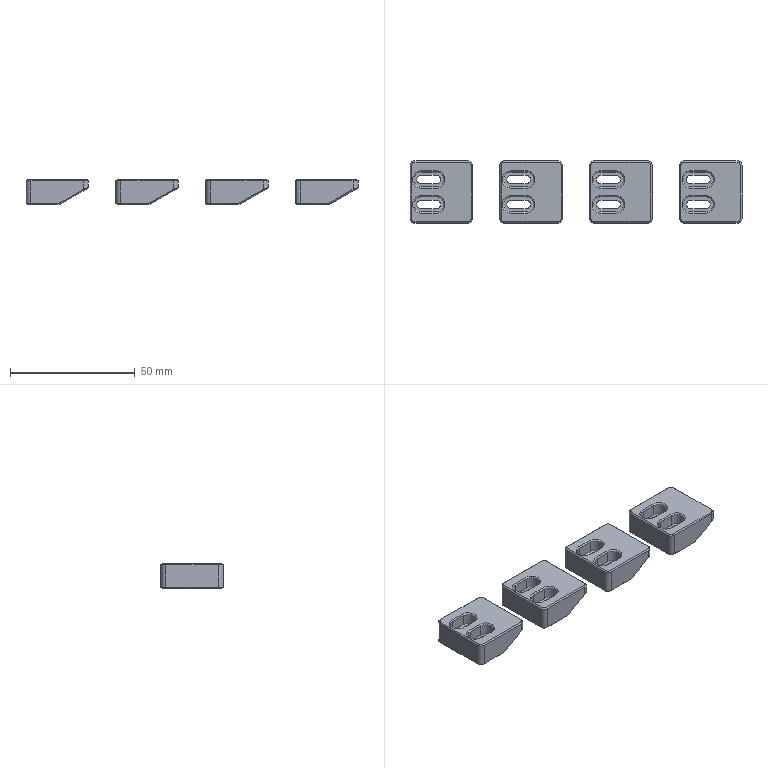NC program | NX | posted with a generic post | part box 133 x 25 x 10 mm
Lines 1 to 18 of 9691:
N10 G17 G21 G94 G90
(FLOOR_WALL , TOOL : D80)
N12 T19 M6
N14 G54
N16 G17 G0 G90 X112.5 Y0. S6500 M3
N18 G43 Z30. H19
N20 Z3.
N22 G94 G1 Z0. F1500.
N24 X109.5
N26 X-109.5
N28 X-112.5
N30 Z3.
N32 G0 Z30.
N34 M5